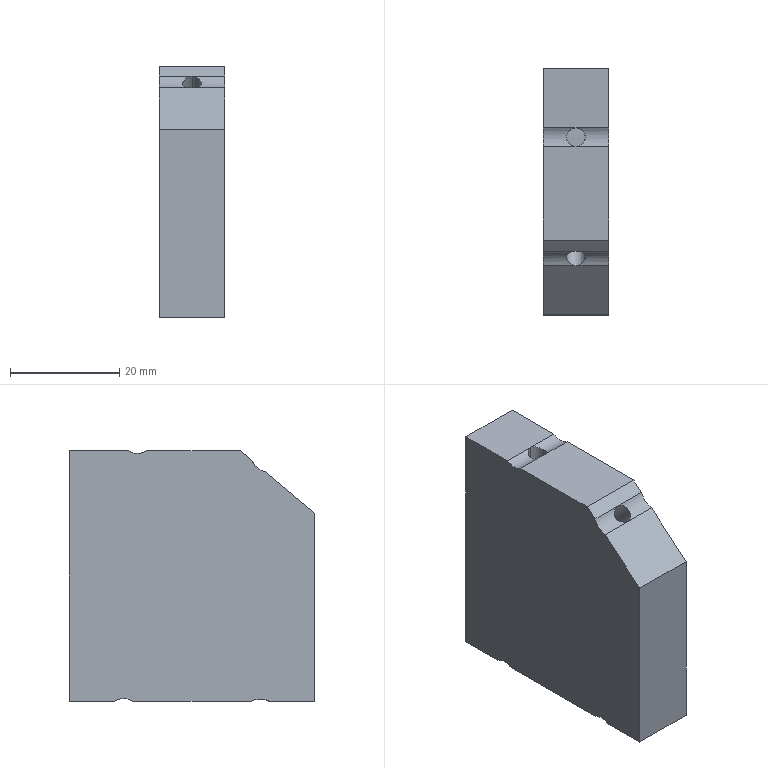Part | SolidWorks | features BaseBody 1 | 1 solid | 33 faces | box 12 x 45 x 45.902 mm | volume 23264 mm3 | cylinder 18 | plane 15 | commonest cylinder face diameters 3.4 x10 5.946 x4 7.056 x4
STEP:
#1=CARTESIAN_POINT('',(-775.626,724.097,383.384));
#2=VERTEX_POINT('',#1);
#3=CARTESIAN_POINT('',(-777.326,725.797,383.384));
#4=VERTEX_POINT('',#3);
#5=CARTESIAN_POINT('',(-775.626,725.797,383.384));
#6=DIRECTION('',(0.000000439,0.,-1.));
#7=DIRECTION('',(-1.,-0.000001546,-0.000000439));
#8=AXIS2_PLACEMENT_3D('',#5,#6,#7);
#9=CIRCLE('',#8,1.7);
#10=EDGE_CURVE('',#2,#4,#9,.T.);
#11=ORIENTED_EDGE('',*,*,#10,.T.);
#12=CARTESIAN_POINT('',(-777.326,725.797,397.85));
#13=VERTEX_POINT('',#12);
#14=CARTESIAN_POINT('',(-777.326,725.797,398.384));
#15=DIRECTION('',(-0.000000439,0.,1.));
#16=VECTOR('',#15,1000.);
#17=LINE('',#14,#16);
#18=EDGE_CURVE('',#4,#13,#17,.T.);
#19=ORIENTED_EDGE('',*,*,#18,.T.);
#20=CARTESIAN_POINT('',(-775.626,724.097,398.384));
#21=VERTEX_POINT('',#20);
#22=CARTESIAN_POINT('',(-777.326,725.797,397.85));
#23=CARTESIAN_POINT('',(-777.326,725.682,397.85));
#24=CARTESIAN_POINT('',(-777.315,725.569,397.856));
#25=CARTESIAN_POINT('',(-777.27,725.348,397.882));
#26=CARTESIAN_POINT('',(-777.236,725.239,397.901));
#27=CARTESIAN_POINT('',(-777.106,724.931,397.971));
#28=CARTESIAN_POINT('',(-776.98,724.746,398.037));
#29=CARTESIAN_POINT('',(-776.673,724.44,398.172));
#30=CARTESIAN_POINT('',(-776.489,724.316,398.243));
#31=CARTESIAN_POINT('',(-776.184,724.187,398.323));
#32=CARTESIAN_POINT('',(-776.075,724.154,398.345));
#33=CARTESIAN_POINT('',(-775.854,724.109,398.375));
#34=CARTESIAN_POINT('',(-775.741,724.097,398.384));
#35=CARTESIAN_POINT('',(-775.626,724.097,398.384));
#36=B_SPLINE_CURVE_WITH_KNOTS('',3,(#22,#23,#24,#25,#26,#27,#28,#29,#30,#31,#32,#33,#34,#35),.UNSPECIFIED.,.F.,.F.,(4,2,2,2,2,2,4),(0.002719,0.003059,0.003399,0.004078,0.004758,0.005097,0.005437),.UNSPECIFIED.);
#37=EDGE_CURVE('',#13,#21,#36,.T.);
#38=ORIENTED_EDGE('',*,*,#37,.T.);
#39=CARTESIAN_POINT('',(-775.626,724.097,383.384));
#40=DIRECTION('',(-0.000000429,0.000000001,1.));
#41=VECTOR('',#40,1000.);
#42=LINE('',#39,#41);
#43=EDGE_CURVE('',#2,#21,#42,.T.);
#44=ORIENTED_EDGE('',*,*,#43,.F.);
#45=EDGE_LOOP('',(#11,#19,#38,#44));
#46=FACE_OUTER_BOUND('',#45,.T.);
#47=CARTESIAN_POINT('',(-775.626,725.797,398.384));
#48=DIRECTION('',(-0.000000439,0.,1.));
#49=DIRECTION('',(-1.,-0.000001544,-0.000000439));
#50=AXIS2_PLACEMENT_3D('',#47,#48,#49);
#51=CYLINDRICAL_SURFACE('',#50,1.7);
#52=ADVANCED_FACE('',(#46),#51,.F.);
#53=CARTESIAN_POINT('',(-777.326,713.226,384.074));
#54=VERTEX_POINT('',#53);
#55=CARTESIAN_POINT('',(-775.626,714.528,385.167));
#56=VERTEX_POINT('',#55);
#57=CARTESIAN_POINT('',(-775.626,713.226,384.074));
#58=DIRECTION('',(-0.000000993,0.6428,-0.766));
#59=DIRECTION('',(-0.000001183,0.766,0.6428));
#60=AXIS2_PLACEMENT_3D('',#57,#58,#59);
#61=CIRCLE('',#60,1.7);
#62=EDGE_CURVE('',#54,#56,#61,.T.);
#63=ORIENTED_EDGE('',*,*,#62,.T.);
#64=CARTESIAN_POINT('',(-775.626,704.886,396.657));
#65=VERTEX_POINT('',#64);
#66=CARTESIAN_POINT('',(-775.626,704.886,396.657));
#67=DIRECTION('',(0.000000993,-0.6428,0.766));
#68=VECTOR('',#67,1000.);
#69=LINE('',#66,#68);
#70=EDGE_CURVE('',#56,#65,#69,.T.);
#71=ORIENTED_EDGE('',*,*,#70,.T.);
#72=CARTESIAN_POINT('',(-777.326,703.865,395.23));
#73=VERTEX_POINT('',#72);
#74=CARTESIAN_POINT('',(-775.626,704.886,396.657));
#75=CARTESIAN_POINT('',(-775.741,704.886,396.657));
#76=CARTESIAN_POINT('',(-775.852,704.882,396.645));
#77=CARTESIAN_POINT('',(-776.072,704.863,396.599));
#78=CARTESIAN_POINT('',(-776.181,704.849,396.564));
#79=CARTESIAN_POINT('',(-776.488,704.791,396.432));
#80=CARTESIAN_POINT('',(-776.673,704.732,396.307));
#81=CARTESIAN_POINT('',(-776.982,704.568,396.023));
#82=CARTESIAN_POINT('',(-777.108,704.461,395.862));
#83=CARTESIAN_POINT('',(-777.237,704.263,395.62));
#84=CARTESIAN_POINT('',(-777.27,704.19,395.538));
#85=CARTESIAN_POINT('',(-777.315,704.035,395.38));
#86=CARTESIAN_POINT('',(-777.326,703.952,395.304));
#87=CARTESIAN_POINT('',(-777.326,703.865,395.23));
#88=B_SPLINE_CURVE_WITH_KNOTS('',3,(#74,#75,#76,#77,#78,#79,#80,#81,#82,#83,#84,#85,#86,#87),.UNSPECIFIED.,.F.,.F.,(4,2,2,2,2,2,4),(0.,0.0003373,0.0006746,0.001349,0.002024,0.002361,0.002699),.UNSPECIFIED.);
#89=EDGE_CURVE('',#65,#73,#88,.T.);
#90=ORIENTED_EDGE('',*,*,#89,.T.);
#91=CARTESIAN_POINT('',(-777.326,703.865,395.23));
#92=DIRECTION('',(-0.000000993,0.6428,-0.766));
#93=VECTOR('',#92,1000.);
#94=LINE('',#91,#93);
#95=EDGE_CURVE('',#73,#54,#94,.T.);
#96=ORIENTED_EDGE('',*,*,#95,.T.);
#97=EDGE_LOOP('',(#63,#71,#90,#96));
#98=FACE_OUTER_BOUND('',#97,.T.);
#99=CARTESIAN_POINT('',(-775.626,703.584,395.565));
#100=DIRECTION('',(0.000000993,-0.6428,0.766));
#101=DIRECTION('',(-0.000001183,0.766,0.6428));
#102=AXIS2_PLACEMENT_3D('',#99,#100,#101);
#103=CYLINDRICAL_SURFACE('',#102,1.7);
#104=ADVANCED_FACE('',(#98),#103,.F.);
#105=CARTESIAN_POINT('',(-777.33,703.297,367.482));
#106=VERTEX_POINT('',#105);
#107=CARTESIAN_POINT('',(-777.33,703.297,352.918));
#108=VERTEX_POINT('',#107);
#109=CARTESIAN_POINT('',(-777.33,703.297,367.482));
#110=DIRECTION('',(0.,0.,-1.));
#111=VECTOR('',#110,1000.);
#112=LINE('',#109,#111);
#113=EDGE_CURVE('',#106,#108,#112,.T.);
#114=ORIENTED_EDGE('',*,*,#113,.F.);
#115=CARTESIAN_POINT('',(-773.93,703.297,367.482));
#116=VERTEX_POINT('',#115);
#117=CARTESIAN_POINT('',(-775.63,703.297,367.482));
#118=DIRECTION('',(0.,0.,1.));
#119=DIRECTION('',(-1.,-0.000001544,0.));
#120=AXIS2_PLACEMENT_3D('',#117,#118,#119);
#121=CIRCLE('',#120,1.7);
#122=EDGE_CURVE('',#106,#116,#121,.T.);
#123=ORIENTED_EDGE('',*,*,#122,.T.);
#124=CARTESIAN_POINT('',(-773.93,703.297,352.918));
#125=VERTEX_POINT('',#124);
#126=CARTESIAN_POINT('',(-773.93,703.297,352.918));
#127=DIRECTION('',(0.,0.,1.));
#128=VECTOR('',#127,1000.);
#129=LINE('',#126,#128);
#130=EDGE_CURVE('',#125,#116,#129,.T.);
#131=ORIENTED_EDGE('',*,*,#130,.F.);
#132=CARTESIAN_POINT('',(-775.63,701.597,352.482));
#133=VERTEX_POINT('',#132);
#134=CARTESIAN_POINT('',(-775.63,701.597,352.482));
#135=CARTESIAN_POINT('',(-775.516,701.597,352.482));
#136=CARTESIAN_POINT('',(-775.404,701.608,352.488));
#137=CARTESIAN_POINT('',(-775.184,701.653,352.512));
#138=CARTESIAN_POINT('',(-775.076,701.686,352.529));
#139=CARTESIAN_POINT('',(-774.769,701.815,352.593));
#140=CARTESIAN_POINT('',(-774.583,701.94,352.651));
#141=CARTESIAN_POINT('',(-774.274,702.248,352.763));
#142=CARTESIAN_POINT('',(-774.148,702.435,352.818));
#143=CARTESIAN_POINT('',(-774.02,702.741,352.876));
#144=CARTESIAN_POINT('',(-773.986,702.85,352.892));
#145=CARTESIAN_POINT('',(-773.941,703.071,352.913));
#146=CARTESIAN_POINT('',(-773.93,703.183,352.918));
#147=CARTESIAN_POINT('',(-773.93,703.297,352.918));
#148=B_SPLINE_CURVE_WITH_KNOTS('',3,(#134,#135,#136,#137,#138,#139,#140,#141,#142,#143,#144,#145,#146,#147),.UNSPECIFIED.,.F.,.F.,(4,2,2,2,2,2,4),(0.000000003,0.0003373,0.0006746,0.001349,0.002024,0.002361,0.002699),.UNSPECIFIED.);
#149=EDGE_CURVE('',#133,#125,#148,.T.);
#150=ORIENTED_EDGE('',*,*,#149,.F.);
#151=CARTESIAN_POINT('',(-777.33,703.297,352.918));
#152=CARTESIAN_POINT('',(-777.33,703.183,352.918));
#153=CARTESIAN_POINT('',(-777.319,703.071,352.913));
#154=CARTESIAN_POINT('',(-777.274,702.851,352.892));
#155=CARTESIAN_POINT('',(-777.241,702.742,352.876));
#156=CARTESIAN_POINT('',(-777.112,702.434,352.818));
#157=CARTESIAN_POINT('',(-776.986,702.248,352.763));
#158=CARTESIAN_POINT('',(-776.677,701.94,352.651));
#159=CARTESIAN_POINT('',(-776.491,701.815,352.593));
#160=CARTESIAN_POINT('',(-776.186,701.687,352.53));
#161=CARTESIAN_POINT('',(-776.077,701.653,352.512));
#162=CARTESIAN_POINT('',(-775.857,701.608,352.488));
#163=CARTESIAN_POINT('',(-775.744,701.597,352.482));
#164=CARTESIAN_POINT('',(-775.63,701.597,352.482));
#165=B_SPLINE_CURVE_WITH_KNOTS('',3,(#151,#152,#153,#154,#155,#156,#157,#158,#159,#160,#161,#162,#163,#164),.UNSPECIFIED.,.F.,.F.,(4,2,2,2,2,2,4),(0.,0.0003374,0.0006747,0.001349,0.002024,0.002362,0.002699),.UNSPECIFIED.);
#166=EDGE_CURVE('',#108,#133,#165,.T.);
#167=ORIENTED_EDGE('',*,*,#166,.F.);
#168=EDGE_LOOP('',(#114,#123,#131,#150,#167));
#169=FACE_OUTER_BOUND('',#168,.T.);
#170=CARTESIAN_POINT('',(-775.63,703.297,352.482));
#171=DIRECTION('',(0.,0.,-1.));
#172=DIRECTION('',(1.,0.000001544,0.));
#173=AXIS2_PLACEMENT_3D('',#170,#171,#172);
#174=CYLINDRICAL_SURFACE('',#173,1.7);
#175=ADVANCED_FACE('',(#169),#174,.F.);
#176=CARTESIAN_POINT('',(-781.626,701.597,352.482));
#177=VERTEX_POINT('',#176);
#178=CARTESIAN_POINT('',(-781.626,704.997,352.482));
#179=VERTEX_POINT('',#178);
#180=CARTESIAN_POINT('',(-781.626,703.297,349.391));
#181=DIRECTION('',(-1.,-0.000002068,-0.000000439));
#182=DIRECTION('',(0.000000612,-0.4819,0.8762));
#183=AXIS2_PLACEMENT_3D('',#180,#181,#182);
#184=CIRCLE('',#183,3.528);
#185=EDGE_CURVE('',#177,#179,#184,.T.);
#186=ORIENTED_EDGE('',*,*,#185,.T.);
#187=CARTESIAN_POINT('',(-775.63,704.997,352.482));
#188=VERTEX_POINT('',#187);
#189=CARTESIAN_POINT('',(-775.63,704.997,352.482));
#190=DIRECTION('',(-1.,-0.000002272,-0.000000153));
#191=VECTOR('',#190,1000.);
#192=LINE('',#189,#191);
#193=EDGE_CURVE('',#188,#179,#192,.T.);
#194=ORIENTED_EDGE('',*,*,#193,.F.);
#195=CARTESIAN_POINT('',(-777.33,703.297,352.918));
#196=CARTESIAN_POINT('',(-777.33,703.411,352.918));
#197=CARTESIAN_POINT('',(-777.319,703.523,352.913));
#198=CARTESIAN_POINT('',(-777.274,703.743,352.892));
#199=CARTESIAN_POINT('',(-777.241,703.852,352.876));
#200=CARTESIAN_POINT('',(-777.112,704.16,352.818));
#201=CARTESIAN_POINT('',(-776.986,704.346,352.763));
#202=CARTESIAN_POINT('',(-776.677,704.654,352.651));
#203=CARTESIAN_POINT('',(-776.491,704.779,352.593));
#204=CARTESIAN_POINT('',(-776.186,704.907,352.53));
#205=CARTESIAN_POINT('',(-776.077,704.941,352.512));
#206=CARTESIAN_POINT('',(-775.857,704.986,352.488));
#207=CARTESIAN_POINT('',(-775.744,704.997,352.482));
#208=CARTESIAN_POINT('',(-775.63,704.997,352.482));
#209=B_SPLINE_CURVE_WITH_KNOTS('',3,(#195,#196,#197,#198,#199,#200,#201,#202,#203,#204,#205,#206,#207,#208),.UNSPECIFIED.,.F.,.F.,(4,2,2,2,2,2,4),(0.,0.0003374,0.0006747,0.001349,0.002024,0.002362,0.002699),.UNSPECIFIED.);
#210=EDGE_CURVE('',#108,#188,#209,.T.);
#211=ORIENTED_EDGE('',*,*,#210,.F.);
#212=ORIENTED_EDGE('',*,*,#166,.T.);
#213=CARTESIAN_POINT('',(-781.626,701.597,352.482));
#214=DIRECTION('',(1.,0.000001661,0.000000159));
#215=VECTOR('',#214,1000.);
#216=LINE('',#213,#215);
#217=EDGE_CURVE('',#177,#133,#216,.T.);
#218=ORIENTED_EDGE('',*,*,#217,.F.);
#219=EDGE_LOOP('',(#186,#194,#211,#212,#218));
#220=FACE_OUTER_BOUND('',#219,.T.);
#221=CARTESIAN_POINT('',(-769.626,703.297,349.391));
#222=DIRECTION('',(1.,0.000002068,0.000000439));
#223=DIRECTION('',(0.000002068,-1.,0.));
#224=AXIS2_PLACEMENT_3D('',#221,#222,#223);
#225=CYLINDRICAL_SURFACE('',#224,3.528);
#226=ADVANCED_FACE('',(#220),#225,.F.);
#227=CARTESIAN_POINT('',(-769.626,693.297,352.482));
#228=VERTEX_POINT('',#227);
#229=CARTESIAN_POINT('',(-769.626,701.597,352.482));
#230=VERTEX_POINT('',#229);
#231=CARTESIAN_POINT('',(-769.626,693.297,352.482));
#232=DIRECTION('',(-0.000001845,1.,-0.000000031));
#233=VECTOR('',#232,1000.);
#234=LINE('',#231,#233);
#235=EDGE_CURVE('',#228,#230,#234,.T.);
#236=ORIENTED_EDGE('',*,*,#235,.F.);
#237=CARTESIAN_POINT('',(-781.626,693.297,352.482));
#238=VERTEX_POINT('',#237);
#239=CARTESIAN_POINT('',(-781.626,693.297,352.482));
#240=DIRECTION('',(1.,0.00000185,0.000000202));
#241=VECTOR('',#240,1000.);
#242=LINE('',#239,#241);
#243=EDGE_CURVE('',#238,#228,#242,.T.);
#244=ORIENTED_EDGE('',*,*,#243,.F.);
#245=CARTESIAN_POINT('',(-781.626,701.597,352.482));
#246=DIRECTION('',(0.000001845,-1.,-0.000000031));
#247=VECTOR('',#246,1000.);
#248=LINE('',#245,#247);
#249=EDGE_CURVE('',#177,#238,#248,.T.);
#250=ORIENTED_EDGE('',*,*,#249,.F.);
#251=ORIENTED_EDGE('',*,*,#217,.T.);
#252=CARTESIAN_POINT('',(-775.63,701.597,352.482));
#253=DIRECTION('',(1.,0.000001668,0.00000016));
#254=VECTOR('',#253,1000.);
#255=LINE('',#252,#254);
#256=EDGE_CURVE('',#133,#230,#255,.T.);
#257=ORIENTED_EDGE('',*,*,#256,.T.);
#258=EDGE_LOOP('',(#236,#244,#250,#251,#257));
#259=FACE_OUTER_BOUND('',#258,.T.);
#260=CARTESIAN_POINT('',(-653.13,738.297,352.482));
#261=DIRECTION('',(0.,0.,1.));
#262=DIRECTION('',(-0.000001544,1.,0.));
#263=AXIS2_PLACEMENT_3D('',#260,#261,#262);
#264=PLANE('',#263);
#265=ADVANCED_FACE('',(#259),#264,.F.);
#266=CARTESIAN_POINT('',(-769.626,704.997,352.482));
#267=VERTEX_POINT('',#266);
#268=CARTESIAN_POINT('',(-769.626,704.997,352.482));
#269=DIRECTION('',(-1.,-0.000002279,-0.000000152));
#270=VECTOR('',#269,1000.);
#271=LINE('',#268,#270);
#272=EDGE_CURVE('',#267,#188,#271,.T.);
#273=ORIENTED_EDGE('',*,*,#272,.F.);
#274=CARTESIAN_POINT('',(-769.626,703.297,349.391));
#275=DIRECTION('',(1.,0.000002068,0.000000439));
#276=DIRECTION('',(-0.000001381,0.4819,0.8762));
#277=AXIS2_PLACEMENT_3D('',#274,#275,#276);
#278=CIRCLE('',#277,3.528);
#279=EDGE_CURVE('',#267,#230,#278,.T.);
#280=ORIENTED_EDGE('',*,*,#279,.T.);
#281=ORIENTED_EDGE('',*,*,#256,.F.);
#282=ORIENTED_EDGE('',*,*,#149,.T.);
#283=CARTESIAN_POINT('',(-775.63,704.997,352.482));
#284=CARTESIAN_POINT('',(-775.516,704.997,352.482));
#285=CARTESIAN_POINT('',(-775.404,704.986,352.488));
#286=CARTESIAN_POINT('',(-775.184,704.941,352.512));
#287=CARTESIAN_POINT('',(-775.076,704.908,352.529));
#288=CARTESIAN_POINT('',(-774.769,704.779,352.593));
#289=CARTESIAN_POINT('',(-774.583,704.654,352.651));
#290=CARTESIAN_POINT('',(-774.274,704.346,352.763));
#291=CARTESIAN_POINT('',(-774.148,704.159,352.818));
#292=CARTESIAN_POINT('',(-774.02,703.853,352.876));
#293=CARTESIAN_POINT('',(-773.986,703.745,352.892));
#294=CARTESIAN_POINT('',(-773.941,703.524,352.913));
#295=CARTESIAN_POINT('',(-773.93,703.411,352.918));
#296=CARTESIAN_POINT('',(-773.93,703.297,352.918));
#297=B_SPLINE_CURVE_WITH_KNOTS('',3,(#283,#284,#285,#286,#287,#288,#289,#290,#291,#292,#293,#294,#295,#296),.UNSPECIFIED.,.F.,.F.,(4,2,2,2,2,2,4),(0.000000002,0.0003373,0.0006746,0.001349,0.002024,0.002361,0.002699),.UNSPECIFIED.);
#298=EDGE_CURVE('',#188,#125,#297,.T.);
#299=ORIENTED_EDGE('',*,*,#298,.F.);
#300=EDGE_LOOP('',(#273,#280,#281,#282,#299));
#301=FACE_OUTER_BOUND('',#300,.T.);
#302=CARTESIAN_POINT('',(-769.626,703.297,349.391));
#303=DIRECTION('',(1.,0.000002068,0.000000439));
#304=DIRECTION('',(0.000002068,-1.,0.));
#305=AXIS2_PLACEMENT_3D('',#302,#303,#304);
#306=CYLINDRICAL_SURFACE('',#305,3.528);
#307=ADVANCED_FACE('',(#301),#306,.F.);
#308=ORIENTED_EDGE('',*,*,#130,.T.);
#309=CARTESIAN_POINT('',(-775.63,703.297,367.482));
#310=DIRECTION('',(0.,0.,1.));
#311=DIRECTION('',(1.,0.000001544,0.));
#312=AXIS2_PLACEMENT_3D('',#309,#310,#311);
#313=CIRCLE('',#312,1.7);
#314=EDGE_CURVE('',#116,#106,#313,.T.);
#315=ORIENTED_EDGE('',*,*,#314,.T.);
#316=ORIENTED_EDGE('',*,*,#113,.T.);
#317=ORIENTED_EDGE('',*,*,#210,.T.);
#318=ORIENTED_EDGE('',*,*,#298,.T.);
#319=EDGE_LOOP('',(#308,#315,#316,#317,#318));
#320=FACE_OUTER_BOUND('',#319,.T.);
#321=CARTESIAN_POINT('',(-775.63,703.297,352.482));
#322=DIRECTION('',(0.,0.,-1.));
#323=DIRECTION('',(1.,0.000001544,0.));
#324=AXIS2_PLACEMENT_3D('',#321,#322,#323);
#325=CYLINDRICAL_SURFACE('',#324,1.7);
#326=ADVANCED_FACE('',(#320),#325,.F.);
#327=ORIENTED_EDGE('',*,*,#314,.F.);
#328=ORIENTED_EDGE('',*,*,#122,.F.);
#329=EDGE_LOOP('',(#327,#328));
#330=FACE_OUTER_BOUND('',#329,.T.);
#331=CARTESIAN_POINT('',(-653.129,0.00034,367.482));
#332=DIRECTION('',(0.,0.,-1.));
#333=DIRECTION('',(1.,0.000001544,0.));
#334=AXIS2_PLACEMENT_3D('',#331,#332,#333);
#335=PLANE('',#334);
#336=ADVANCED_FACE('',(#330),#335,.T.);
#337=CARTESIAN_POINT('',(-769.626,693.297,386.933));
#338=VERTEX_POINT('',#337);
#339=CARTESIAN_POINT('',(-769.626,693.297,352.482));
#340=DIRECTION('',(-0.000000416,0.00000003,1.));
#341=VECTOR('',#340,1000.);
#342=LINE('',#339,#341);
#343=EDGE_CURVE('',#228,#338,#342,.T.);
#344=ORIENTED_EDGE('',*,*,#343,.F.);
#345=ORIENTED_EDGE('',*,*,#235,.T.);
#346=ORIENTED_EDGE('',*,*,#279,.F.);
#347=CARTESIAN_POINT('',(-769.626,726.597,352.482));
#348=VERTEX_POINT('',#347);
#349=CARTESIAN_POINT('',(-769.626,704.997,352.482));
#350=DIRECTION('',(-0.000001893,1.,-0.000000006));
#351=VECTOR('',#350,1000.);
#352=LINE('',#349,#351);
#353=EDGE_CURVE('',#267,#348,#352,.T.);
#354=ORIENTED_EDGE('',*,*,#353,.T.);
#355=CARTESIAN_POINT('',(-769.626,729.997,352.482));
#356=VERTEX_POINT('',#355);
#357=CARTESIAN_POINT('',(-769.626,728.297,350.043));
#358=DIRECTION('',(1.,0.000002068,0.000000439));
#359=DIRECTION('',(-0.000001543,0.5718,0.8204));
#360=AXIS2_PLACEMENT_3D('',#357,#358,#359);
#361=CIRCLE('',#360,2.973);
#362=EDGE_CURVE('',#356,#348,#361,.T.);
#363=ORIENTED_EDGE('',*,*,#362,.F.);
#364=CARTESIAN_POINT('',(-769.626,738.297,352.482));
#365=VERTEX_POINT('',#364);
#366=CARTESIAN_POINT('',(-769.626,738.297,352.482));
#367=DIRECTION('',(0.000001845,-1.,-0.00000002));
#368=VECTOR('',#367,1000.);
#369=LINE('',#366,#368);
#370=EDGE_CURVE('',#365,#356,#369,.T.);
#371=ORIENTED_EDGE('',*,*,#370,.F.);
#372=CARTESIAN_POINT('',(-769.626,738.297,398.384));
#373=VERTEX_POINT('',#372);
#374=CARTESIAN_POINT('',(-769.626,738.297,398.384));
#375=DIRECTION('',(0.000000456,-0.000000023,-1.));
#376=VECTOR('',#375,1000.);
#377=LINE('',#374,#376);
#378=EDGE_CURVE('',#373,#365,#377,.T.);
#379=ORIENTED_EDGE('',*,*,#378,.F.);
#380=CARTESIAN_POINT('',(-769.626,727.497,398.384));
#381=VERTEX_POINT('',#380);
#382=CARTESIAN_POINT('',(-769.626,727.497,398.384));
#383=DIRECTION('',(-0.00000203,1.,0.));
#384=VECTOR('',#383,1000.);
#385=LINE('',#382,#384);
#386=EDGE_CURVE('',#381,#373,#385,.T.);
#387=ORIENTED_EDGE('',*,*,#386,.F.);
#388=CARTESIAN_POINT('',(-769.626,724.097,398.384));
#389=VERTEX_POINT('',#388);
#390=CARTESIAN_POINT('',(-769.626,725.797,400.823));
#391=DIRECTION('',(1.,0.000002068,0.000000439));
#392=DIRECTION('',(0.000001543,-0.5718,-0.8204));
#393=AXIS2_PLACEMENT_3D('',#390,#391,#392);
#394=CIRCLE('',#393,2.973);
#395=EDGE_CURVE('',#389,#381,#394,.T.);
#396=ORIENTED_EDGE('',*,*,#395,.F.);
#397=CARTESIAN_POINT('',(-769.626,706.944,398.384));
#398=VERTEX_POINT('',#397);
#399=CARTESIAN_POINT('',(-769.626,706.944,398.384));
#400=DIRECTION('',(-0.000002068,1.,0.));
#401=VECTOR('',#400,1000.);
#402=LINE('',#399,#401);
#403=EDGE_CURVE('',#398,#389,#402,.T.);
#404=ORIENTED_EDGE('',*,*,#403,.F.);
#405=CARTESIAN_POINT('',(-769.626,704.886,396.657));
#406=VERTEX_POINT('',#405);
#407=CARTESIAN_POINT('',(-769.626,704.886,396.657));
#408=DIRECTION('',(-0.000001866,0.766,0.6428));
#409=VECTOR('',#408,1000.);
#410=LINE('',#407,#409);
#411=EDGE_CURVE('',#406,#398,#410,.T.);
#412=ORIENTED_EDGE('',*,*,#411,.F.);
#413=CARTESIAN_POINT('',(-769.626,702.282,394.472));
#414=VERTEX_POINT('',#413);
#415=CARTESIAN_POINT('',(-769.626,701.597,397.933));
#416=DIRECTION('',(1.,0.000002068,0.000000439));
#417=DIRECTION('',(0.000000029,0.1941,-0.981));
#418=AXIS2_PLACEMENT_3D('',#415,#416,#417);
#419=CIRCLE('',#418,3.528);
#420=EDGE_CURVE('',#414,#406,#419,.T.);
#421=ORIENTED_EDGE('',*,*,#420,.F.);
#422=CARTESIAN_POINT('',(-769.626,693.297,386.933));
#423=DIRECTION('',(-0.000001832,0.766,0.6428));
#424=VECTOR('',#423,1000.);
#425=LINE('',#422,#424);
#426=EDGE_CURVE('',#338,#414,#425,.T.);
#427=ORIENTED_EDGE('',*,*,#426,.F.);
#428=EDGE_LOOP('',(#344,#345,#346,#354,#363,#371,#379,#387,#396,#404,#412,#421,#427));
#429=FACE_OUTER_BOUND('',#428,.T.);
#430=CARTESIAN_POINT('',(-769.625,-0.0002426,-0.2503));
#431=DIRECTION('',(-1.,-0.000002068,-0.000000439));
#432=DIRECTION('',(-0.000002068,1.,0.));
#433=AXIS2_PLACEMENT_3D('',#430,#431,#432);
#434=PLANE('',#433);
#435=ADVANCED_FACE('',(#429),#434,.F.);
#436=CARTESIAN_POINT('',(-781.626,693.297,386.933));
#437=VERTEX_POINT('',#436);
#438=CARTESIAN_POINT('',(-769.626,693.297,386.933));
#439=DIRECTION('',(-1.,-0.000002025,-0.000000403));
#440=VECTOR('',#439,1000.);
#441=LINE('',#438,#440);
#442=EDGE_CURVE('',#338,#437,#441,.T.);
#443=ORIENTED_EDGE('',*,*,#442,.F.);
#444=ORIENTED_EDGE('',*,*,#426,.T.);
#445=CARTESIAN_POINT('',(-775.626,702.282,394.472));
#446=VERTEX_POINT('',#445);
#447=CARTESIAN_POINT('',(-769.626,702.282,394.472));
#448=DIRECTION('',(-1.,-0.000002069,-0.000000438));
#449=VECTOR('',#448,1000.);
#450=LINE('',#447,#449);
#451=EDGE_CURVE('',#414,#446,#450,.T.);
#452=ORIENTED_EDGE('',*,*,#451,.T.);
#453=CARTESIAN_POINT('',(-781.626,702.282,394.472));
#454=VERTEX_POINT('',#453);
#455=CARTESIAN_POINT('',(-775.626,702.282,394.472));
#456=DIRECTION('',(-1.,-0.000002067,-0.00000044));
#457=VECTOR('',#456,1000.);
#458=LINE('',#455,#457);
#459=EDGE_CURVE('',#446,#454,#458,.T.);
#460=ORIENTED_EDGE('',*,*,#459,.T.);
#461=CARTESIAN_POINT('',(-781.626,702.282,394.472));
#462=DIRECTION('',(0.000001832,-0.766,-0.6428));
#463=VECTOR('',#462,1000.);
#464=LINE('',#461,#463);
#465=EDGE_CURVE('',#454,#437,#464,.T.);
#466=ORIENTED_EDGE('',*,*,#465,.T.);
#467=EDGE_LOOP('',(#443,#444,#452,#460,#466));
#468=FACE_OUTER_BOUND('',#467,.T.);
#469=CARTESIAN_POINT('',(-781.626,693.297,386.933));
#470=DIRECTION('',(0.000000993,-0.6428,0.766));
#471=DIRECTION('',(0.000001866,-0.766,-0.6428));
#472=AXIS2_PLACEMENT_3D('',#469,#470,#471);
#473=PLANE('',#472);
#474=ADVANCED_FACE('',(#468),#473,.T.);
#475=CARTESIAN_POINT('',(-781.626,724.097,398.384));
#476=VERTEX_POINT('',#475);
#477=CARTESIAN_POINT('',(-781.626,706.944,398.384));
#478=VERTEX_POINT('',#477);
#479=CARTESIAN_POINT('',(-781.626,724.097,398.384));
#480=DIRECTION('',(0.000002068,-1.,0.));
#481=VECTOR('',#480,1000.);
#482=LINE('',#479,#481);
#483=EDGE_CURVE('',#476,#478,#482,.T.);
#484=ORIENTED_EDGE('',*,*,#483,.F.);
#485=CARTESIAN_POINT('',(-781.626,727.497,398.384));
#486=VERTEX_POINT('',#485);
#487=CARTESIAN_POINT('',(-781.626,725.797,400.823));
#488=DIRECTION('',(-1.,-0.000002068,-0.000000439));
#489=DIRECTION('',(-0.000000822,0.5718,-0.8204));
#490=AXIS2_PLACEMENT_3D('',#487,#488,#489);
#491=CIRCLE('',#490,2.973);
#492=EDGE_CURVE('',#486,#476,#491,.T.);
#493=ORIENTED_EDGE('',*,*,#492,.F.);
#494=CARTESIAN_POINT('',(-781.626,738.297,398.384));
#495=VERTEX_POINT('',#494);
#496=CARTESIAN_POINT('',(-781.626,738.297,398.384));
#497=DIRECTION('',(0.00000203,-1.,0.));
#498=VECTOR('',#497,1000.);
#499=LINE('',#496,#498);
#500=EDGE_CURVE('',#495,#486,#499,.T.);
#501=ORIENTED_EDGE('',*,*,#500,.F.);
#502=CARTESIAN_POINT('',(-781.626,738.297,352.482));
#503=VERTEX_POINT('',#502);
#504=CARTESIAN_POINT('',(-781.626,738.297,352.482));
#505=DIRECTION('',(-0.000000456,-0.000000023,1.));
#506=VECTOR('',#505,1000.);
#507=LINE('',#504,#506);
#508=EDGE_CURVE('',#503,#495,#507,.T.);
#509=ORIENTED_EDGE('',*,*,#508,.F.);
#510=CARTESIAN_POINT('',(-781.626,729.997,352.482));
#511=VERTEX_POINT('',#510);
#512=CARTESIAN_POINT('',(-781.626,729.997,352.482));
#513=DIRECTION('',(-0.000001845,1.,-0.000000021));
#514=VECTOR('',#513,1000.);
#515=LINE('',#512,#514);
#516=EDGE_CURVE('',#511,#503,#515,.T.);
#517=ORIENTED_EDGE('',*,*,#516,.F.);
#518=CARTESIAN_POINT('',(-781.626,726.597,352.482));
#519=VERTEX_POINT('',#518);
#520=CARTESIAN_POINT('',(-781.626,728.297,350.043));
#521=DIRECTION('',(-1.,-0.000002068,-0.000000439));
#522=DIRECTION('',(0.000000822,-0.5718,0.8204));
#523=AXIS2_PLACEMENT_3D('',#520,#521,#522);
#524=CIRCLE('',#523,2.973);
#525=EDGE_CURVE('',#519,#511,#524,.T.);
#526=ORIENTED_EDGE('',*,*,#525,.F.);
#527=CARTESIAN_POINT('',(-781.626,726.597,352.482));
#528=DIRECTION('',(0.000001893,-1.,-0.000000005));
#529=VECTOR('',#528,1000.);
#530=LINE('',#527,#529);
#531=EDGE_CURVE('',#519,#179,#530,.T.);
#532=ORIENTED_EDGE('',*,*,#531,.T.);
#533=ORIENTED_EDGE('',*,*,#185,.F.);
#534=ORIENTED_EDGE('',*,*,#249,.T.);
#535=CARTESIAN_POINT('',(-781.626,693.297,386.933));
#536=DIRECTION('',(0.000000416,0.00000003,-1.));
#537=VECTOR('',#536,1000.);
#538=LINE('',#535,#537);
#539=EDGE_CURVE('',#437,#238,#538,.T.);
#540=ORIENTED_EDGE('',*,*,#539,.F.);
#541=ORIENTED_EDGE('',*,*,#465,.F.);
#542=CARTESIAN_POINT('',(-781.626,704.886,396.657));
#543=VERTEX_POINT('',#542);
#544=CARTESIAN_POINT('',(-781.626,701.597,397.933));
#545=DIRECTION('',(-1.,-0.000002068,-0.000000439));
#546=DIRECTION('',(-0.000001769,0.9324,-0.3615));
#547=AXIS2_PLACEMENT_3D('',#544,#545,#546);
#548=CIRCLE('',#547,3.528);
#549=EDGE_CURVE('',#543,#454,#548,.T.);
#550=ORIENTED_EDGE('',*,*,#549,.F.);
#551=CARTESIAN_POINT('',(-781.626,706.944,398.384));
#552=DIRECTION('',(0.000001866,-0.766,-0.6428));
#553=VECTOR('',#552,1000.);
#554=LINE('',#551,#553);
#555=EDGE_CURVE('',#478,#543,#554,.T.);
#556=ORIENTED_EDGE('',*,*,#555,.F.);
#557=EDGE_LOOP('',(#484,#493,#501,#509,#517,#526,#532,#533,#534,#540,#541,#550,#556));
#558=FACE_OUTER_BOUND('',#557,.T.);
#559=CARTESIAN_POINT('',(-781.625,-0.0002674,-0.2503));
#560=DIRECTION('',(-1.,-0.000002068,-0.000000439));
#561=DIRECTION('',(-0.000002068,1.,0.));
#562=AXIS2_PLACEMENT_3D('',#559,#560,#561);
#563=PLANE('',#562);
#564=ADVANCED_FACE('',(#558),#563,.T.);
#565=ORIENTED_EDGE('',*,*,#411,.T.);
#566=CARTESIAN_POINT('',(-769.626,706.944,398.384));
#567=DIRECTION('',(-1.,-0.000002068,-0.000000439));
#568=VECTOR('',#567,1000.);
#569=LINE('',#566,#568);
#570=EDGE_CURVE('',#398,#478,#569,.T.);
#571=ORIENTED_EDGE('',*,*,#570,.T.);
#572=ORIENTED_EDGE('',*,*,#555,.T.);
#573=CARTESIAN_POINT('',(-781.626,704.886,396.657));
#574=DIRECTION('',(1.,0.000002068,0.000000439));
#575=VECTOR('',#574,1000.);
#576=LINE('',#573,#575);
#577=EDGE_CURVE('',#543,#65,#576,.T.);
#578=ORIENTED_EDGE('',*,*,#577,.T.);
#579=CARTESIAN_POINT('',(-775.626,704.886,396.657));
#580=DIRECTION('',(1.,0.000002068,0.000000439));
#581=VECTOR('',#580,1000.);
#582=LINE('',#579,#581);
#583=EDGE_CURVE('',#65,#406,#582,.T.);
#584=ORIENTED_EDGE('',*,*,#583,.T.);
#585=EDGE_LOOP('',(#565,#571,#572,#578,#584));
#586=FACE_OUTER_BOUND('',#585,.T.);
#587=CARTESIAN_POINT('',(-781.626,693.297,386.933));
#588=DIRECTION('',(0.000000993,-0.6428,0.766));
#589=DIRECTION('',(0.000001866,-0.766,-0.6428));
#590=AXIS2_PLACEMENT_3D('',#587,#588,#589);
#591=PLANE('',#590);
#592=ADVANCED_FACE('',(#586),#591,.T.);
#593=ORIENTED_EDGE('',*,*,#420,.T.);
#594=ORIENTED_EDGE('',*,*,#583,.F.);
#595=CARTESIAN_POINT('',(-773.926,703.865,395.23));
#596=VERTEX_POINT('',#595);
#597=CARTESIAN_POINT('',(-773.926,703.865,395.23));
#598=CARTESIAN_POINT('',(-773.926,703.952,395.304));
#599=CARTESIAN_POINT('',(-773.938,704.034,395.38));
#600=CARTESIAN_POINT('',(-773.982,704.189,395.537));
#601=CARTESIAN_POINT('',(-774.016,704.262,395.619));
#602=CARTESIAN_POINT('',(-774.145,704.461,395.862));
#603=CARTESIAN_POINT('',(-774.271,704.568,396.023));
#604=CARTESIAN_POINT('',(-774.579,704.732,396.307));
#605=CARTESIAN_POINT('',(-774.765,704.791,396.432));
#606=CARTESIAN_POINT('',(-775.071,704.849,396.563));
#607=CARTESIAN_POINT('',(-775.179,704.863,396.598));
#608=CARTESIAN_POINT('',(-775.4,704.882,396.645));
#609=CARTESIAN_POINT('',(-775.512,704.886,396.657));
#610=CARTESIAN_POINT('',(-775.626,704.886,396.657));
#611=B_SPLINE_CURVE_WITH_KNOTS('',3,(#597,#598,#599,#600,#601,#602,#603,#604,#605,#606,#607,#608,#609,#610),.UNSPECIFIED.,.F.,.F.,(4,2,2,2,2,2,4),(0.,0.0003374,0.0006748,0.00135,0.002024,0.002362,0.002699),.UNSPECIFIED.);
#612=EDGE_CURVE('',#596,#65,#611,.T.);
#613=ORIENTED_EDGE('',*,*,#612,.F.);
#614=CARTESIAN_POINT('',(-775.626,702.282,394.472));
#615=CARTESIAN_POINT('',(-775.512,702.282,394.472));
#616=CARTESIAN_POINT('',(-775.4,702.295,394.474));
#617=CARTESIAN_POINT('',(-775.181,702.344,394.485));
#618=CARTESIAN_POINT('',(-775.072,702.381,394.493));
#619=CARTESIAN_POINT('',(-774.765,702.52,394.526));
#620=CARTESIAN_POINT('',(-774.579,702.653,394.563));
#621=CARTESIAN_POINT('',(-774.271,702.961,394.675));
#622=CARTESIAN_POINT('',(-774.145,703.139,394.753));
#623=CARTESIAN_POINT('',(-774.016,703.411,394.905));
#624=CARTESIAN_POINT('',(-773.982,703.505,394.963));
#625=CARTESIAN_POINT('',(-773.938,703.688,395.089));
#626=CARTESIAN_POINT('',(-773.926,703.777,395.157));
#627=CARTESIAN_POINT('',(-773.926,703.865,395.23));
#628=B_SPLINE_CURVE_WITH_KNOTS('',3,(#614,#615,#616,#617,#618,#619,#620,#621,#622,#623,#624,#625,#626,#627),.UNSPECIFIED.,.F.,.F.,(4,2,2,2,2,2,4),(0.,0.0003373,0.0006746,0.001349,0.002024,0.002361,0.002699),.UNSPECIFIED.);
#629=EDGE_CURVE('',#446,#596,#628,.T.);
#630=ORIENTED_EDGE('',*,*,#629,.F.);
#631=ORIENTED_EDGE('',*,*,#451,.F.);
#632=EDGE_LOOP('',(#593,#594,#613,#630,#631));
#633=FACE_OUTER_BOUND('',#632,.T.);
#634=CARTESIAN_POINT('',(-769.626,701.597,397.933));
#635=DIRECTION('',(1.,0.000002068,0.000000439));
#636=DIRECTION('',(0.000002068,-1.,0.));
#637=AXIS2_PLACEMENT_3D('',#634,#635,#636);
#638=CYLINDRICAL_SURFACE('',#637,3.528);
#639=ADVANCED_FACE('',(#633),#638,.F.);
#640=CARTESIAN_POINT('',(-773.926,713.226,384.074));
#641=VERTEX_POINT('',#640);
#642=CARTESIAN_POINT('',(-773.926,713.226,384.074));
#643=DIRECTION('',(0.000000993,-0.6428,0.766));
#644=VECTOR('',#643,1000.);
#645=LINE('',#642,#644);
#646=EDGE_CURVE('',#641,#596,#645,.T.);
#647=ORIENTED_EDGE('',*,*,#646,.F.);
#648=CARTESIAN_POINT('',(-775.626,713.226,384.074));
#649=DIRECTION('',(-0.000000993,0.6428,-0.766));
#650=DIRECTION('',(0.000001183,-0.766,-0.6428));
#651=AXIS2_PLACEMENT_3D('',#648,#649,#650);
#652=CIRCLE('',#651,1.7);
#653=EDGE_CURVE('',#641,#54,#652,.T.);
#654=ORIENTED_EDGE('',*,*,#653,.T.);
#655=ORIENTED_EDGE('',*,*,#95,.F.);
#656=CARTESIAN_POINT('',(-775.626,702.282,394.472));
#657=CARTESIAN_POINT('',(-775.741,702.282,394.472));
#658=CARTESIAN_POINT('',(-775.852,702.295,394.474));
#659=CARTESIAN_POINT('',(-776.072,702.344,394.485));
#660=CARTESIAN_POINT('',(-776.181,702.381,394.493));
#661=CARTESIAN_POINT('',(-776.488,702.52,394.526));
#662=CARTESIAN_POINT('',(-776.673,702.653,394.563));
#663=CARTESIAN_POINT('',(-776.982,702.961,394.675));
#664=CARTESIAN_POINT('',(-777.108,703.139,394.753));
#665=CARTESIAN_POINT('',(-777.237,703.411,394.905));
#666=CARTESIAN_POINT('',(-777.27,703.505,394.963));
#667=CARTESIAN_POINT('',(-777.315,703.688,395.089));
#668=CARTESIAN_POINT('',(-777.326,703.777,395.157));
#669=CARTESIAN_POINT('',(-777.326,703.865,395.23));
#670=B_SPLINE_CURVE_WITH_KNOTS('',3,(#656,#657,#658,#659,#660,#661,#662,#663,#664,#665,#666,#667,#668,#669),.UNSPECIFIED.,.F.,.F.,(4,2,2,2,2,2,4),(0.,0.0003373,0.0006746,0.001349,0.002024,0.002361,0.002699),.UNSPECIFIED.);
#671=EDGE_CURVE('',#446,#73,#670,.T.);
#672=ORIENTED_EDGE('',*,*,#671,.F.);
#673=ORIENTED_EDGE('',*,*,#629,.T.);
#674=EDGE_LOOP('',(#647,#654,#655,#672,#673));
#675=FACE_OUTER_BOUND('',#674,.T.);
#676=CARTESIAN_POINT('',(-775.626,703.584,395.565));
#677=DIRECTION('',(0.000000993,-0.6428,0.766));
#678=DIRECTION('',(-0.000001183,0.766,0.6428));
#679=AXIS2_PLACEMENT_3D('',#676,#677,#678);
#680=CYLINDRICAL_SURFACE('',#679,1.7);
#681=ADVANCED_FACE('',(#675),#680,.F.);
#682=ORIENTED_EDGE('',*,*,#671,.T.);
#683=ORIENTED_EDGE('',*,*,#89,.F.);
#684=ORIENTED_EDGE('',*,*,#577,.F.);
#685=ORIENTED_EDGE('',*,*,#549,.T.);
#686=ORIENTED_EDGE('',*,*,#459,.F.);
#687=EDGE_LOOP('',(#682,#683,#684,#685,#686));
#688=FACE_OUTER_BOUND('',#687,.T.);
#689=CARTESIAN_POINT('',(-769.626,701.597,397.933));
#690=DIRECTION('',(1.,0.000002068,0.000000439));
#691=DIRECTION('',(0.000002068,-1.,0.));
#692=AXIS2_PLACEMENT_3D('',#689,#690,#691);
#693=CYLINDRICAL_SURFACE('',#692,3.528);
#694=ADVANCED_FACE('',(#688),#693,.F.);
#695=ORIENTED_EDGE('',*,*,#70,.F.);
#696=CARTESIAN_POINT('',(-775.626,713.226,384.074));
#697=DIRECTION('',(-0.000000993,0.6428,-0.766));
#698=DIRECTION('',(-0.000001183,0.766,0.6428));
#699=AXIS2_PLACEMENT_3D('',#696,#697,#698);
#700=CIRCLE('',#699,1.7);
#701=EDGE_CURVE('',#56,#641,#700,.T.);
#702=ORIENTED_EDGE('',*,*,#701,.T.);
#703=ORIENTED_EDGE('',*,*,#646,.T.);
#704=ORIENTED_EDGE('',*,*,#612,.T.);
#705=EDGE_LOOP('',(#695,#702,#703,#704));
#706=FACE_OUTER_BOUND('',#705,.T.);
#707=CARTESIAN_POINT('',(-775.626,703.584,395.565));
#708=DIRECTION('',(0.000000993,-0.6428,0.766));
#709=DIRECTION('',(-0.000001183,0.766,0.6428));
#710=AXIS2_PLACEMENT_3D('',#707,#708,#709);
#711=CYLINDRICAL_SURFACE('',#710,1.7);
#712=ADVANCED_FACE('',(#706),#711,.F.);
#713=ORIENTED_EDGE('',*,*,#653,.F.);
#714=ORIENTED_EDGE('',*,*,#701,.F.);
#715=ORIENTED_EDGE('',*,*,#62,.F.);
#716=EDGE_LOOP('',(#713,#714,#715));
#717=FACE_OUTER_BOUND('',#716,.T.);
#718=CARTESIAN_POINT('',(-653.129,105.445,-125.914));
#719=DIRECTION('',(0.000000993,-0.6428,0.766));
#720=DIRECTION('',(-1.,-0.000001544,0.));
#721=AXIS2_PLACEMENT_3D('',#718,#719,#720);
#722=PLANE('',#721);
#723=ADVANCED_FACE('',(#717),#722,.T.);
#724=ORIENTED_EDGE('',*,*,#570,.F.);
#725=ORIENTED_EDGE('',*,*,#403,.T.);
#726=CARTESIAN_POINT('',(-769.626,724.097,398.384));
#727=DIRECTION('',(-1.,-0.000002068,-0.000000439));
#728=VECTOR('',#727,1000.);
#729=LINE('',#726,#728);
#730=EDGE_CURVE('',#389,#21,#729,.T.);
#731=ORIENTED_EDGE('',*,*,#730,.T.);
#732=CARTESIAN_POINT('',(-775.626,724.097,398.384));
#733=DIRECTION('',(-1.,-0.000002068,-0.000000439));
#734=VECTOR('',#733,1000.);
#735=LINE('',#732,#734);
#736=EDGE_CURVE('',#21,#476,#735,.T.);
#737=ORIENTED_EDGE('',*,*,#736,.T.);
#738=ORIENTED_EDGE('',*,*,#483,.T.);
#739=EDGE_LOOP('',(#724,#725,#731,#737,#738));
#740=FACE_OUTER_BOUND('',#739,.T.);
#741=CARTESIAN_POINT('',(-781.626,706.944,398.384));
#742=DIRECTION('',(-0.000000439,0.,1.));
#743=DIRECTION('',(0.000002068,-1.,0.));
#744=AXIS2_PLACEMENT_3D('',#741,#742,#743);
#745=PLANE('',#744);
#746=ADVANCED_FACE('',(#740),#745,.T.);
#747=ORIENTED_EDGE('',*,*,#736,.F.);
#748=ORIENTED_EDGE('',*,*,#37,.F.);
#749=CARTESIAN_POINT('',(-775.626,727.497,398.384));
#750=VERTEX_POINT('',#749);
#751=CARTESIAN_POINT('',(-775.626,727.497,398.384));
#752=CARTESIAN_POINT('',(-775.741,727.497,398.384));
#753=CARTESIAN_POINT('',(-775.854,727.485,398.376));
#754=CARTESIAN_POINT('',(-776.074,727.441,398.345));
#755=CARTESIAN_POINT('',(-776.183,727.407,398.323));
#756=CARTESIAN_POINT('',(-776.489,727.278,398.243));
#757=CARTESIAN_POINT('',(-776.673,727.154,398.172));
#758=CARTESIAN_POINT('',(-776.904,726.924,398.07));
#759=CARTESIAN_POINT('',(-776.974,726.839,398.037));
#760=CARTESIAN_POINT('',(-777.097,726.657,397.975));
#761=CARTESIAN_POINT('',(-777.149,726.561,397.948));
#762=CARTESIAN_POINT('',(-777.235,726.356,397.901));
#763=CARTESIAN_POINT('',(-777.269,726.247,397.882));
#764=CARTESIAN_POINT('',(-777.315,726.025,397.856));
#765=CARTESIAN_POINT('',(-777.326,725.912,397.85));
#766=CARTESIAN_POINT('',(-777.326,725.797,397.85));
#767=B_SPLINE_CURVE_WITH_KNOTS('',3,(#751,#752,#753,#754,#755,#756,#757,#758,#759,#760,#761,#762,#763,#764,#765,#766),.UNSPECIFIED.,.F.,.F.,(4,2,2,2,2,2,2,4),(0.,0.0003399,0.0006798,0.00136,0.0017,0.002039,0.002379,0.002719),.UNSPECIFIED.);
#768=EDGE_CURVE('',#750,#13,#767,.T.);
#769=ORIENTED_EDGE('',*,*,#768,.F.);
#770=CARTESIAN_POINT('',(-781.626,727.497,398.384));
#771=DIRECTION('',(1.,0.000002068,0.000000439));
#772=VECTOR('',#771,1000.);
#773=LINE('',#770,#772);
#774=EDGE_CURVE('',#486,#750,#773,.T.);
#775=ORIENTED_EDGE('',*,*,#774,.F.);
#776=ORIENTED_EDGE('',*,*,#492,.T.);
#777=EDGE_LOOP('',(#747,#748,#769,#775,#776));
#778=FACE_OUTER_BOUND('',#777,.T.);
#779=CARTESIAN_POINT('',(-769.626,725.797,400.823));
#780=DIRECTION('',(1.,0.000002068,0.000000439));
#781=DIRECTION('',(0.000002068,-1.,0.));
#782=AXIS2_PLACEMENT_3D('',#779,#780,#781);
#783=CYLINDRICAL_SURFACE('',#782,2.973);
#784=ADVANCED_FACE('',(#778),#783,.F.);
#785=ORIENTED_EDGE('',*,*,#386,.T.);
#786=CARTESIAN_POINT('',(-769.626,738.297,398.384));
#787=DIRECTION('',(-1.,-0.000002025,-0.000000439));
#788=VECTOR('',#787,1000.);
#789=LINE('',#786,#788);
#790=EDGE_CURVE('',#373,#495,#789,.T.);
#791=ORIENTED_EDGE('',*,*,#790,.T.);
#792=ORIENTED_EDGE('',*,*,#500,.T.);
#793=ORIENTED_EDGE('',*,*,#774,.T.);
#794=CARTESIAN_POINT('',(-775.626,727.497,398.384));
#795=DIRECTION('',(1.,0.000002068,0.000000439));
#796=VECTOR('',#795,1000.);
#797=LINE('',#794,#796);
#798=EDGE_CURVE('',#750,#381,#797,.T.);
#799=ORIENTED_EDGE('',*,*,#798,.T.);
#800=EDGE_LOOP('',(#785,#791,#792,#793,#799));
#801=FACE_OUTER_BOUND('',#800,.T.);
#802=CARTESIAN_POINT('',(-781.626,706.944,398.384));
#803=DIRECTION('',(-0.000000439,0.,1.));
#804=DIRECTION('',(0.000002068,-1.,0.));
#805=AXIS2_PLACEMENT_3D('',#802,#803,#804);
#806=PLANE('',#805);
#807=ADVANCED_FACE('',(#801),#806,.T.);
#808=ORIENTED_EDGE('',*,*,#395,.T.);
#809=ORIENTED_EDGE('',*,*,#798,.F.);
#810=CARTESIAN_POINT('',(-775.626,727.497,398.384));
#811=CARTESIAN_POINT('',(-775.511,727.497,398.384));
#812=CARTESIAN_POINT('',(-775.398,727.485,398.376));
#813=CARTESIAN_POINT('',(-775.178,727.441,398.345));
#814=CARTESIAN_POINT('',(-775.069,727.407,398.323));
#815=CARTESIAN_POINT('',(-774.763,727.278,398.243));
#816=CARTESIAN_POINT('',(-774.579,727.154,398.172));
#817=CARTESIAN_POINT('',(-774.349,726.924,398.07));
#818=CARTESIAN_POINT('',(-774.279,726.839,398.037));
#819=CARTESIAN_POINT('',(-774.156,726.657,397.975));
#820=CARTESIAN_POINT('',(-774.104,726.561,397.948));
#821=CARTESIAN_POINT('',(-774.017,726.357,397.901));
#822=CARTESIAN_POINT('',(-773.983,726.247,397.882));
#823=CARTESIAN_POINT('',(-773.938,726.026,397.856));
#824=CARTESIAN_POINT('',(-773.926,725.913,397.85));
#825=CARTESIAN_POINT('',(-773.926,725.683,397.85));
#826=CARTESIAN_POINT('',(-773.938,725.57,397.856));
#827=CARTESIAN_POINT('',(-773.982,725.349,397.882));
#828=CARTESIAN_POINT('',(-774.016,725.239,397.901));
#829=CARTESIAN_POINT('',(-774.146,724.931,397.971));
#830=CARTESIAN_POINT('',(-774.272,724.746,398.037));
#831=CARTESIAN_POINT('',(-774.58,724.44,398.172));
#832=CARTESIAN_POINT('',(-774.763,724.316,398.243));
#833=CARTESIAN_POINT('',(-775.068,724.187,398.323));
#834=CARTESIAN_POINT('',(-775.177,724.154,398.345));
#835=CARTESIAN_POINT('',(-775.398,724.109,398.375));
#836=CARTESIAN_POINT('',(-775.511,724.097,398.384));
#837=CARTESIAN_POINT('',(-775.626,724.097,398.384));
#838=B_SPLINE_CURVE_WITH_KNOTS('',3,(#810,#811,#812,#813,#814,#815,#816,#817,#818,#819,#820,#821,#822,#823,#824,#825,#826,#827,#828,#829,#830,#831,#832,#833,#834,#835,#836,#837),.UNSPECIFIED.,.F.,.F.,(4,2,2,2,2,2,2,2,2,2,2,2,2,4),(-0.002722,-0.002382,-0.002042,-0.001361,-0.001021,-0.000681,-0.0003409,-0.000000756,0.0003394,0.0006795,0.00136,0.00204,0.00238,0.00272),.UNSPECIFIED.);
#839=EDGE_CURVE('',#750,#21,#838,.T.);
#840=ORIENTED_EDGE('',*,*,#839,.T.);
#841=ORIENTED_EDGE('',*,*,#730,.F.);
#842=EDGE_LOOP('',(#808,#809,#840,#841));
#843=FACE_OUTER_BOUND('',#842,.T.);
#844=CARTESIAN_POINT('',(-769.626,725.797,400.823));
#845=DIRECTION('',(1.,0.000002068,0.000000439));
#846=DIRECTION('',(0.000002068,-1.,0.));
#847=AXIS2_PLACEMENT_3D('',#844,#845,#846);
#848=CYLINDRICAL_SURFACE('',#847,2.973);
#849=ADVANCED_FACE('',(#843),#848,.F.);
#850=CARTESIAN_POINT('',(-775.626,727.497,383.384));
#851=VERTEX_POINT('',#850);
#852=CARTESIAN_POINT('',(-775.626,727.497,398.384));
#853=DIRECTION('',(0.000000449,0.000000001,-1.));
#854=VECTOR('',#853,1000.);
#855=LINE('',#852,#854);
#856=EDGE_CURVE('',#750,#851,#855,.T.);
#857=ORIENTED_EDGE('',*,*,#856,.T.);
#858=CARTESIAN_POINT('',(-775.626,725.797,383.384));
#859=DIRECTION('',(0.000000439,0.,-1.));
#860=DIRECTION('',(1.,0.000001546,0.000000439));
#861=AXIS2_PLACEMENT_3D('',#858,#859,#860);
#862=CIRCLE('',#861,1.7);
#863=EDGE_CURVE('',#851,#2,#862,.T.);
#864=ORIENTED_EDGE('',*,*,#863,.T.);
#865=ORIENTED_EDGE('',*,*,#43,.T.);
#866=ORIENTED_EDGE('',*,*,#839,.F.);
#867=EDGE_LOOP('',(#857,#864,#865,#866));
#868=FACE_OUTER_BOUND('',#867,.T.);
#869=CARTESIAN_POINT('',(-775.626,725.797,398.384));
#870=DIRECTION('',(-0.000000439,0.,1.));
#871=DIRECTION('',(-1.,-0.000001544,-0.000000439));
#872=AXIS2_PLACEMENT_3D('',#869,#870,#871);
#873=CYLINDRICAL_SURFACE('',#872,1.7);
#874=ADVANCED_FACE('',(#868),#873,.F.);
#875=ORIENTED_EDGE('',*,*,#18,.F.);
#876=CARTESIAN_POINT('',(-775.626,725.797,383.384));
#877=DIRECTION('',(0.000000439,0.,-1.));
#878=DIRECTION('',(-1.,-0.000001546,-0.000000439));
#879=AXIS2_PLACEMENT_3D('',#876,#877,#878);
#880=CIRCLE('',#879,1.7);
#881=EDGE_CURVE('',#4,#851,#880,.T.);
#882=ORIENTED_EDGE('',*,*,#881,.T.);
#883=ORIENTED_EDGE('',*,*,#856,.F.);
#884=ORIENTED_EDGE('',*,*,#768,.T.);
#885=EDGE_LOOP('',(#875,#882,#883,#884));
#886=FACE_OUTER_BOUND('',#885,.T.);
#887=CARTESIAN_POINT('',(-775.626,725.797,398.384));
#888=DIRECTION('',(-0.000000439,0.,1.));
#889=DIRECTION('',(-1.,-0.000001544,-0.000000439));
#890=AXIS2_PLACEMENT_3D('',#887,#888,#889);
#891=CYLINDRICAL_SURFACE('',#890,1.7);
#892=ADVANCED_FACE('',(#886),#891,.F.);
#893=ORIENTED_EDGE('',*,*,#10,.F.);
#894=ORIENTED_EDGE('',*,*,#863,.F.);
#895=ORIENTED_EDGE('',*,*,#881,.F.);
#896=EDGE_LOOP('',(#893,#894,#895));
#897=FACE_OUTER_BOUND('',#896,.T.);
#898=CARTESIAN_POINT('',(-781.625,-0.0002674,383.384));
#899=DIRECTION('',(-0.000000439,0.,1.));
#900=DIRECTION('',(-1.,-0.000001544,-0.000000439));
#901=AXIS2_PLACEMENT_3D('',#898,#899,#900);
#902=PLANE('',#901);
#903=ADVANCED_FACE('',(#897),#902,.T.);
#904=ORIENTED_EDGE('',*,*,#790,.F.);
#905=ORIENTED_EDGE('',*,*,#378,.T.);
#906=CARTESIAN_POINT('',(-769.626,738.297,352.482));
#907=DIRECTION('',(-1.,-0.00000185,-0.000000204));
#908=VECTOR('',#907,1000.);
#909=LINE('',#906,#908);
#910=EDGE_CURVE('',#365,#503,#909,.T.);
#911=ORIENTED_EDGE('',*,*,#910,.T.);
#912=ORIENTED_EDGE('',*,*,#508,.T.);
#913=EDGE_LOOP('',(#904,#905,#911,#912));
#914=FACE_OUTER_BOUND('',#913,.T.);
#915=CARTESIAN_POINT('',(-781.626,738.297,398.384));
#916=DIRECTION('',(-0.000002068,1.,0.));
#917=DIRECTION('',(-0.000000439,0.,1.));
#918=AXIS2_PLACEMENT_3D('',#915,#916,#917);
#919=PLANE('',#918);
#920=ADVANCED_FACE('',(#914),#919,.T.);
#921=ORIENTED_EDGE('',*,*,#910,.F.);
#922=ORIENTED_EDGE('',*,*,#370,.T.);
#923=CARTESIAN_POINT('',(-775.63,729.997,352.482));
#924=VERTEX_POINT('',#923);
#925=CARTESIAN_POINT('',(-769.626,729.997,352.482));
#926=DIRECTION('',(-1.,-0.000002186,-0.000000176));
#927=VECTOR('',#926,1000.);
#928=LINE('',#925,#927);
#929=EDGE_CURVE('',#356,#924,#928,.T.);
#930=ORIENTED_EDGE('',*,*,#929,.T.);
#931=CARTESIAN_POINT('',(-775.63,729.997,352.482));
#932=DIRECTION('',(-1.,-0.000002169,-0.000000177));
#933=VECTOR('',#932,1000.);
#934=LINE('',#931,#933);
#935=EDGE_CURVE('',#924,#511,#934,.T.);
#936=ORIENTED_EDGE('',*,*,#935,.T.);
#937=ORIENTED_EDGE('',*,*,#516,.T.);
#938=EDGE_LOOP('',(#921,#922,#930,#936,#937));
#939=FACE_OUTER_BOUND('',#938,.T.);
#940=CARTESIAN_POINT('',(-653.13,738.297,352.482));
#941=DIRECTION('',(0.,0.,1.));
#942=DIRECTION('',(-1.,-0.000001544,0.));
#943=AXIS2_PLACEMENT_3D('',#940,#941,#942);
#944=PLANE('',#943);
#945=ADVANCED_FACE('',(#939),#944,.F.);
#946=CARTESIAN_POINT('',(-777.33,728.297,353.016));
#947=VERTEX_POINT('',#946);
#948=CARTESIAN_POINT('',(-777.33,728.297,353.016));
#949=CARTESIAN_POINT('',(-777.33,728.412,353.016));
#950=CARTESIAN_POINT('',(-777.318,728.525,353.009));
#951=CARTESIAN_POINT('',(-777.274,728.746,352.984));
#952=CARTESIAN_POINT('',(-777.24,728.855,352.965));
#953=CARTESIAN_POINT('',(-777.11,729.163,352.895));
#954=CARTESIAN_POINT('',(-776.984,729.348,352.829));
#955=CARTESIAN_POINT('',(-776.676,729.654,352.693));
#956=CARTESIAN_POINT('',(-776.493,729.778,352.622));
#957=CARTESIAN_POINT('',(-776.188,729.907,352.543));
#958=CARTESIAN_POINT('',(-776.079,729.941,352.52));
#959=CARTESIAN_POINT('',(-775.858,729.985,352.49));
#960=CARTESIAN_POINT('',(-775.745,729.997,352.482));
#961=CARTESIAN_POINT('',(-775.63,729.997,352.482));
#962=B_SPLINE_CURVE_WITH_KNOTS('',3,(#948,#949,#950,#951,#952,#953,#954,#955,#956,#957,#958,#959,#960,#961),.UNSPECIFIED.,.F.,.F.,(4,2,2,2,2,2,4),(0.,0.00034,0.0006801,0.00136,0.00204,0.00238,0.00272),.UNSPECIFIED.);
#963=EDGE_CURVE('',#947,#924,#962,.T.);
#964=ORIENTED_EDGE('',*,*,#963,.F.);
#965=CARTESIAN_POINT('',(-775.63,726.597,352.482));
#966=VERTEX_POINT('',#965);
#967=CARTESIAN_POINT('',(-775.63,726.597,352.482));
#968=CARTESIAN_POINT('',(-775.745,726.597,352.482));
#969=CARTESIAN_POINT('',(-775.858,726.609,352.49));
#970=CARTESIAN_POINT('',(-776.078,726.653,352.52));
#971=CARTESIAN_POINT('',(-776.187,726.687,352.543));
#972=CARTESIAN_POINT('',(-776.493,726.816,352.622));
#973=CARTESIAN_POINT('',(-776.677,726.94,352.693));
#974=CARTESIAN_POINT('',(-776.907,727.17,352.795));
#975=CARTESIAN_POINT('',(-776.978,727.255,352.829));
#976=CARTESIAN_POINT('',(-777.101,727.437,352.89));
#977=CARTESIAN_POINT('',(-777.153,727.533,352.918));
#978=CARTESIAN_POINT('',(-777.239,727.738,352.965));
#979=CARTESIAN_POINT('',(-777.273,727.847,352.984));
#980=CARTESIAN_POINT('',(-777.318,728.069,353.009));
#981=CARTESIAN_POINT('',(-777.33,728.182,353.016));
#982=CARTESIAN_POINT('',(-777.33,728.297,353.016));
#983=B_SPLINE_CURVE_WITH_KNOTS('',3,(#967,#968,#969,#970,#971,#972,#973,#974,#975,#976,#977,#978,#979,#980,#981,#982),.UNSPECIFIED.,.F.,.F.,(4,2,2,2,2,2,2,4),(0.,0.0003399,0.0006798,0.00136,0.0017,0.002039,0.002379,0.002719),.UNSPECIFIED.);
#984=EDGE_CURVE('',#966,#947,#983,.T.);
#985=ORIENTED_EDGE('',*,*,#984,.F.);
#986=CARTESIAN_POINT('',(-781.626,726.597,352.482));
#987=DIRECTION('',(1.,0.00000168,0.000000134));
#988=VECTOR('',#987,1000.);
#989=LINE('',#986,#988);
#990=EDGE_CURVE('',#519,#966,#989,.T.);
#991=ORIENTED_EDGE('',*,*,#990,.F.);
#992=ORIENTED_EDGE('',*,*,#525,.T.);
#993=ORIENTED_EDGE('',*,*,#935,.F.);
#994=EDGE_LOOP('',(#964,#985,#991,#992,#993));
#995=FACE_OUTER_BOUND('',#994,.T.);
#996=CARTESIAN_POINT('',(-769.626,728.297,350.043));
#997=DIRECTION('',(1.,0.000002068,0.000000439));
#998=DIRECTION('',(0.000002068,-1.,0.));
#999=AXIS2_PLACEMENT_3D('',#996,#997,#998);
#1000=CYLINDRICAL_SURFACE('',#999,2.973);
#1001=ADVANCED_FACE('',(#995),#1000,.F.);
#1002=ORIENTED_EDGE('',*,*,#990,.T.);
#1003=CARTESIAN_POINT('',(-775.63,726.597,352.482));
#1004=DIRECTION('',(1.,0.000001688,0.000000135));
#1005=VECTOR('',#1004,1000.);
#1006=LINE('',#1003,#1005);
#1007=EDGE_CURVE('',#966,#348,#1006,.T.);
#1008=ORIENTED_EDGE('',*,*,#1007,.T.);
#1009=ORIENTED_EDGE('',*,*,#353,.F.);
#1010=ORIENTED_EDGE('',*,*,#272,.T.);
#1011=ORIENTED_EDGE('',*,*,#193,.T.);
#1012=ORIENTED_EDGE('',*,*,#531,.F.);
#1013=EDGE_LOOP('',(#1002,#1008,#1009,#1010,#1011,#1012));
#1014=FACE_OUTER_BOUND('',#1013,.T.);
#1015=CARTESIAN_POINT('',(-653.13,738.297,352.482));
#1016=DIRECTION('',(0.,0.,1.));
#1017=DIRECTION('',(-1.,-0.000001544,0.));
#1018=AXIS2_PLACEMENT_3D('',#1015,#1016,#1017);
#1019=PLANE('',#1018);
#1020=ADVANCED_FACE('',(#1014),#1019,.F.);
#1021=ORIENTED_EDGE('',*,*,#362,.T.);
#1022=ORIENTED_EDGE('',*,*,#1007,.F.);
#1023=CARTESIAN_POINT('',(-773.93,728.297,353.016));
#1024=VERTEX_POINT('',#1023);
#1025=CARTESIAN_POINT('',(-775.63,726.597,352.482));
#1026=CARTESIAN_POINT('',(-775.515,726.597,352.482));
#1027=CARTESIAN_POINT('',(-775.402,726.609,352.49));
#1028=CARTESIAN_POINT('',(-775.182,726.653,352.52));
#1029=CARTESIAN_POINT('',(-775.073,726.687,352.543));
#1030=CARTESIAN_POINT('',(-774.767,726.816,352.622));
#1031=CARTESIAN_POINT('',(-774.583,726.94,352.693));
#1032=CARTESIAN_POINT('',(-774.353,727.17,352.795));
#1033=CARTESIAN_POINT('',(-774.282,727.255,352.829));
#1034=CARTESIAN_POINT('',(-774.16,727.437,352.89));
#1035=CARTESIAN_POINT('',(-774.107,727.533,352.918));
#1036=CARTESIAN_POINT('',(-774.021,727.738,352.965));
#1037=CARTESIAN_POINT('',(-773.987,727.847,352.984));
#1038=CARTESIAN_POINT('',(-773.942,728.069,353.009));
#1039=CARTESIAN_POINT('',(-773.93,728.182,353.016));
#1040=CARTESIAN_POINT('',(-773.93,728.297,353.016));
#1041=B_SPLINE_CURVE_WITH_KNOTS('',3,(#1025,#1026,#1027,#1028,#1029,#1030,#1031,#1032,#1033,#1034,#1035,#1036,#1037,#1038,#1039,#1040),.UNSPECIFIED.,.F.,.F.,(4,2,2,2,2,2,2,4),(0.000000003,0.0003399,0.0006798,0.00136,0.0017,0.00204,0.002379,0.002719),.UNSPECIFIED.);
#1042=EDGE_CURVE('',#966,#1024,#1041,.T.);
#1043=ORIENTED_EDGE('',*,*,#1042,.T.);
#1044=CARTESIAN_POINT('',(-775.63,729.997,352.482));
#1045=CARTESIAN_POINT('',(-775.515,729.997,352.482));
#1046=CARTESIAN_POINT('',(-775.402,729.985,352.49));
#1047=CARTESIAN_POINT('',(-775.182,729.941,352.52));
#1048=CARTESIAN_POINT('',(-775.073,729.907,352.543));
#1049=CARTESIAN_POINT('',(-774.767,729.778,352.622));
#1050=CARTESIAN_POINT('',(-774.583,729.654,352.693));
#1051=CARTESIAN_POINT('',(-774.353,729.424,352.795));
#1052=CARTESIAN_POINT('',(-774.282,729.339,352.829));
#1053=CARTESIAN_POINT('',(-774.16,729.157,352.89));
#1054=CARTESIAN_POINT('',(-774.107,729.061,352.918));
#1055=CARTESIAN_POINT('',(-774.021,728.856,352.965));
#1056=CARTESIAN_POINT('',(-773.987,728.747,352.984));
#1057=CARTESIAN_POINT('',(-773.942,728.525,353.009));
#1058=CARTESIAN_POINT('',(-773.93,728.412,353.016));
#1059=CARTESIAN_POINT('',(-773.93,728.297,353.016));
#1060=B_SPLINE_CURVE_WITH_KNOTS('',3,(#1044,#1045,#1046,#1047,#1048,#1049,#1050,#1051,#1052,#1053,#1054,#1055,#1056,#1057,#1058,#1059),.UNSPECIFIED.,.F.,.F.,(4,2,2,2,2,2,2,4),(0.000000003,0.0003399,0.0006798,0.00136,0.0017,0.00204,0.002379,0.002719),.UNSPECIFIED.);
#1061=EDGE_CURVE('',#924,#1024,#1060,.T.);
#1062=ORIENTED_EDGE('',*,*,#1061,.F.);
#1063=ORIENTED_EDGE('',*,*,#929,.F.);
#1064=EDGE_LOOP('',(#1021,#1022,#1043,#1062,#1063));
#1065=FACE_OUTER_BOUND('',#1064,.T.);
#1066=CARTESIAN_POINT('',(-769.626,728.297,350.043));
#1067=DIRECTION('',(1.,0.000002068,0.000000439));
#1068=DIRECTION('',(0.000002068,-1.,0.));
#1069=AXIS2_PLACEMENT_3D('',#1066,#1067,#1068);
#1070=CYLINDRICAL_SURFACE('',#1069,2.973);
#1071=ADVANCED_FACE('',(#1065),#1070,.F.);
#1072=CARTESIAN_POINT('',(-773.93,728.297,367.482));
#1073=VERTEX_POINT('',#1072);
#1074=CARTESIAN_POINT('',(-773.93,728.297,353.016));
#1075=DIRECTION('',(0.,0.,1.));
#1076=VECTOR('',#1075,1000.);
#1077=LINE('',#1074,#1076);
#1078=EDGE_CURVE('',#1024,#1073,#1077,.T.);
#1079=ORIENTED_EDGE('',*,*,#1078,.T.);
#1080=CARTESIAN_POINT('',(-777.33,728.297,367.482));
#1081=VERTEX_POINT('',#1080);
#1082=CARTESIAN_POINT('',(-775.63,728.297,367.482));
#1083=DIRECTION('',(0.,0.,1.));
#1084=DIRECTION('',(1.,0.000001544,0.));
#1085=AXIS2_PLACEMENT_3D('',#1082,#1083,#1084);
#1086=CIRCLE('',#1085,1.7);
#1087=EDGE_CURVE('',#1073,#1081,#1086,.T.);
#1088=ORIENTED_EDGE('',*,*,#1087,.T.);
#1089=CARTESIAN_POINT('',(-777.33,728.297,367.482));
#1090=DIRECTION('',(0.,0.,-1.));
#1091=VECTOR('',#1090,1000.);
#1092=LINE('',#1089,#1091);
#1093=EDGE_CURVE('',#1081,#947,#1092,.T.);
#1094=ORIENTED_EDGE('',*,*,#1093,.T.);
#1095=ORIENTED_EDGE('',*,*,#963,.T.);
#1096=ORIENTED_EDGE('',*,*,#1061,.T.);
#1097=EDGE_LOOP('',(#1079,#1088,#1094,#1095,#1096));
#1098=FACE_OUTER_BOUND('',#1097,.T.);
#1099=CARTESIAN_POINT('',(-775.63,728.297,352.482));
#1100=DIRECTION('',(0.,0.,-1.));
#1101=DIRECTION('',(1.,0.000001544,0.));
#1102=AXIS2_PLACEMENT_3D('',#1099,#1100,#1101);
#1103=CYLINDRICAL_SURFACE('',#1102,1.7);
#1104=ADVANCED_FACE('',(#1098),#1103,.F.);
#1105=ORIENTED_EDGE('',*,*,#1093,.F.);
#1106=CARTESIAN_POINT('',(-775.63,728.297,367.482));
#1107=DIRECTION('',(0.,0.,1.));
#1108=DIRECTION('',(-1.,-0.000001544,0.));
#1109=AXIS2_PLACEMENT_3D('',#1106,#1107,#1108);
#1110=CIRCLE('',#1109,1.7);
#1111=EDGE_CURVE('',#1081,#1073,#1110,.T.);
#1112=ORIENTED_EDGE('',*,*,#1111,.T.);
#1113=ORIENTED_EDGE('',*,*,#1078,.F.);
#1114=ORIENTED_EDGE('',*,*,#1042,.F.);
#1115=ORIENTED_EDGE('',*,*,#984,.T.);
#1116=EDGE_LOOP('',(#1105,#1112,#1113,#1114,#1115));
#1117=FACE_OUTER_BOUND('',#1116,.T.);
#1118=CARTESIAN_POINT('',(-775.63,728.297,352.482));
#1119=DIRECTION('',(0.,0.,-1.));
#1120=DIRECTION('',(1.,0.000001544,0.));
#1121=AXIS2_PLACEMENT_3D('',#1118,#1119,#1120);
#1122=CYLINDRICAL_SURFACE('',#1121,1.7);
#1123=ADVANCED_FACE('',(#1117),#1122,.F.);
#1124=ORIENTED_EDGE('',*,*,#1087,.F.);
#1125=ORIENTED_EDGE('',*,*,#1111,.F.);
#1126=EDGE_LOOP('',(#1124,#1125));
#1127=FACE_OUTER_BOUND('',#1126,.T.);
#1128=CARTESIAN_POINT('',(-653.129,0.00034,367.482));
#1129=DIRECTION('',(0.,0.,-1.));
#1130=DIRECTION('',(1.,0.000001544,0.));
#1131=AXIS2_PLACEMENT_3D('',#1128,#1129,#1130);
#1132=PLANE('',#1131);
#1133=ADVANCED_FACE('',(#1127),#1132,.T.);
#1134=ORIENTED_EDGE('',*,*,#442,.T.);
#1135=ORIENTED_EDGE('',*,*,#539,.T.);
#1136=ORIENTED_EDGE('',*,*,#243,.T.);
#1137=ORIENTED_EDGE('',*,*,#343,.T.);
#1138=EDGE_LOOP('',(#1134,#1135,#1136,#1137));
#1139=FACE_OUTER_BOUND('',#1138,.T.);
#1140=CARTESIAN_POINT('',(-781.626,693.297,342.482));
#1141=DIRECTION('',(0.000002068,-1.,0.));
#1142=DIRECTION('',(0.000000439,0.,-1.));
#1143=AXIS2_PLACEMENT_3D('',#1140,#1141,#1142);
#1144=PLANE('',#1143);
#1145=ADVANCED_FACE('',(#1139),#1144,.T.);
#1146=CLOSED_SHELL('',(#52,#104,#175,#226,#265,#307,#326,#336,#435,#474,#564,#592,#639,#681,#694,#712,#723,#746,#784,#807,#849,#874,#892,#903,#920,#945,#1001,#1020,#1071,#1104,#1123,#1133,#1145));
#1147=MANIFOLD_SOLID_BREP('',#1146);
#1148=CARTESIAN_POINT('',(0.,0.,0.));
#1149=DIRECTION('',(0.,0.,1.));
#1150=DIRECTION('',(1.,0.,0.));
#1151=AXIS2_PLACEMENT_3D('',#1148,#1149,#1150);
#1152=(LENGTH_UNIT()NAMED_UNIT(*)SI_UNIT(.MILLI.,.METRE.));
#1153=UNCERTAINTY_MEASURE_WITH_UNIT(LENGTH_MEASURE(0.00001),#1152,'','');
#1154=(NAMED_UNIT(*)PLANE_ANGLE_UNIT()SI_UNIT($,.RADIAN.));
#1155=(NAMED_UNIT(*)SI_UNIT($,.STERADIAN.)SOLID_ANGLE_UNIT());
#1156=(GEOMETRIC_REPRESENTATION_CONTEXT(3)GLOBAL_UNCERTAINTY_ASSIGNED_CONTEXT((#1153))GLOBAL_UNIT_ASSIGNED_CONTEXT((#1152,#1154,#1155))REPRESENTATION_CONTEXT('',''));
#1157=ADVANCED_BREP_SHAPE_REPRESENTATION('',(#1147,#1151),#1156);